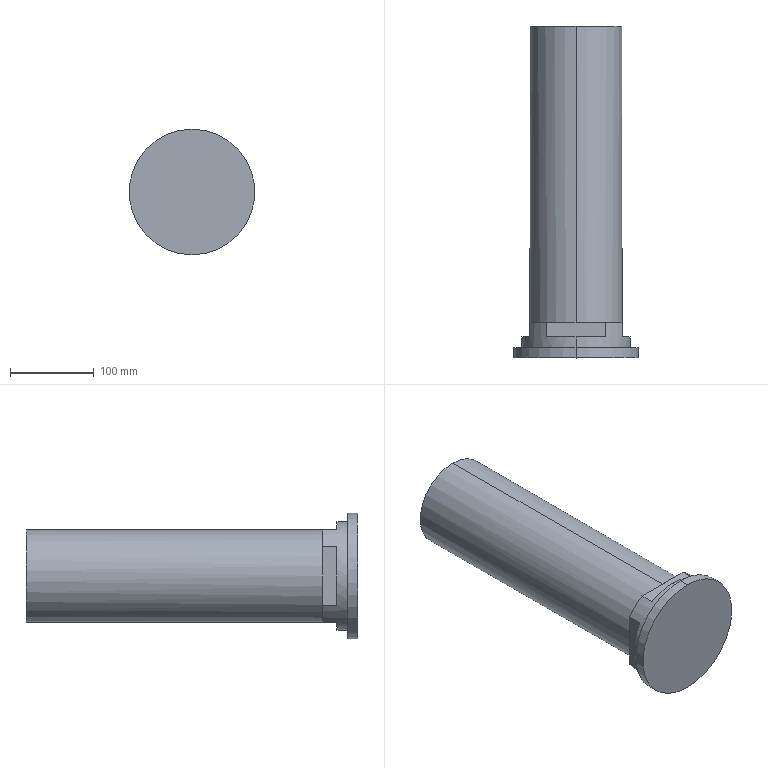Part | SolidWorks | features ICE 4, BaseBody 1 | 1 solid | 21 faces | box 150 x 396 x 150 mm | volume 3942504 mm3 | plane 15 | cylinder 6 | commonest cylinder face diameters 110 x2 130 x2 150 x2
STEP:
#1=CARTESIAN_POINT('',(0.,25.,65.));
#2=VERTEX_POINT('',#1);
#3=CARTESIAN_POINT('',(34.641,25.,55.));
#4=VERTEX_POINT('',#3);
#5=CARTESIAN_POINT('',(0.,25.,0.));
#6=DIRECTION('',(0.,1.,0.));
#7=DIRECTION('',(0.,0.,1.));
#8=AXIS2_PLACEMENT_3D('',#5,#6,#7);
#9=CIRCLE('',#8,65.);
#10=EDGE_CURVE('',#2,#4,#9,.T.);
#11=ORIENTED_EDGE('',*,*,#10,.F.);
#12=CARTESIAN_POINT('',(0.,12.,65.));
#13=VERTEX_POINT('',#12);
#14=CARTESIAN_POINT('',(0.,208.848,65.));
#15=DIRECTION('',(0.,-1.,0.));
#16=VECTOR('',#15,1000.);
#17=LINE('',#14,#16);
#18=EDGE_CURVE('',#2,#13,#17,.T.);
#19=ORIENTED_EDGE('',*,*,#18,.T.);
#20=CARTESIAN_POINT('',(0.,12.,-65.));
#21=VERTEX_POINT('',#20);
#22=CARTESIAN_POINT('',(0.,12.,0.));
#23=DIRECTION('',(0.,1.,0.));
#24=DIRECTION('',(0.,0.,1.));
#25=AXIS2_PLACEMENT_3D('',#22,#23,#24);
#26=CIRCLE('',#25,65.);
#27=EDGE_CURVE('',#13,#21,#26,.T.);
#28=ORIENTED_EDGE('',*,*,#27,.T.);
#29=CARTESIAN_POINT('',(0.,25.,-65.));
#30=VERTEX_POINT('',#29);
#31=CARTESIAN_POINT('',(0.,208.848,-65.));
#32=DIRECTION('',(0.,-1.,0.));
#33=VECTOR('',#32,1000.);
#34=LINE('',#31,#33);
#35=EDGE_CURVE('',#30,#21,#34,.T.);
#36=ORIENTED_EDGE('',*,*,#35,.F.);
#37=CARTESIAN_POINT('',(34.641,25.,-55.));
#38=VERTEX_POINT('',#37);
#39=CARTESIAN_POINT('',(0.,25.,0.));
#40=DIRECTION('',(0.,1.,0.));
#41=DIRECTION('',(0.,0.,1.));
#42=AXIS2_PLACEMENT_3D('',#39,#40,#41);
#43=CIRCLE('',#42,65.);
#44=EDGE_CURVE('',#38,#30,#43,.T.);
#45=ORIENTED_EDGE('',*,*,#44,.F.);
#46=CARTESIAN_POINT('',(34.641,42.,-55.));
#47=VERTEX_POINT('',#46);
#48=CARTESIAN_POINT('',(34.641,197.563,-55.));
#49=DIRECTION('',(0.,-1.,0.));
#50=VECTOR('',#49,1000.);
#51=LINE('',#48,#50);
#52=EDGE_CURVE('',#47,#38,#51,.T.);
#53=ORIENTED_EDGE('',*,*,#52,.F.);
#54=CARTESIAN_POINT('',(55.,42.,-34.641));
#55=VERTEX_POINT('',#54);
#56=CARTESIAN_POINT('',(0.,42.,0.));
#57=DIRECTION('',(0.,1.,0.));
#58=DIRECTION('',(0.,0.,1.));
#59=AXIS2_PLACEMENT_3D('',#56,#57,#58);
#60=CIRCLE('',#59,65.);
#61=EDGE_CURVE('',#55,#47,#60,.T.);
#62=ORIENTED_EDGE('',*,*,#61,.F.);
#63=CARTESIAN_POINT('',(55.,25.,-34.641));
#64=VERTEX_POINT('',#63);
#65=CARTESIAN_POINT('',(55.,197.563,-34.641));
#66=DIRECTION('',(0.,-1.,0.));
#67=VECTOR('',#66,1000.);
#68=LINE('',#65,#67);
#69=EDGE_CURVE('',#55,#64,#68,.T.);
#70=ORIENTED_EDGE('',*,*,#69,.T.);
#71=CARTESIAN_POINT('',(55.,25.,34.641));
#72=VERTEX_POINT('',#71);
#73=CARTESIAN_POINT('',(0.,25.,0.));
#74=DIRECTION('',(0.,1.,0.));
#75=DIRECTION('',(0.,0.,1.));
#76=AXIS2_PLACEMENT_3D('',#73,#74,#75);
#77=CIRCLE('',#76,65.);
#78=EDGE_CURVE('',#72,#64,#77,.T.);
#79=ORIENTED_EDGE('',*,*,#78,.F.);
#80=CARTESIAN_POINT('',(55.,42.,34.641));
#81=VERTEX_POINT('',#80);
#82=CARTESIAN_POINT('',(55.,197.563,34.641));
#83=DIRECTION('',(0.,-1.,0.));
#84=VECTOR('',#83,1000.);
#85=LINE('',#82,#84);
#86=EDGE_CURVE('',#81,#72,#85,.T.);
#87=ORIENTED_EDGE('',*,*,#86,.F.);
#88=CARTESIAN_POINT('',(34.641,42.,55.));
#89=VERTEX_POINT('',#88);
#90=CARTESIAN_POINT('',(0.,42.,0.));
#91=DIRECTION('',(0.,1.,0.));
#92=DIRECTION('',(0.,0.,1.));
#93=AXIS2_PLACEMENT_3D('',#90,#91,#92);
#94=CIRCLE('',#93,65.);
#95=EDGE_CURVE('',#89,#81,#94,.T.);
#96=ORIENTED_EDGE('',*,*,#95,.F.);
#97=CARTESIAN_POINT('',(34.641,197.563,55.));
#98=DIRECTION('',(0.,-1.,0.));
#99=VECTOR('',#98,1000.);
#100=LINE('',#97,#99);
#101=EDGE_CURVE('',#89,#4,#100,.T.);
#102=ORIENTED_EDGE('',*,*,#101,.T.);
#103=EDGE_LOOP('',(#11,#19,#28,#36,#45,#53,#62,#70,#79,#87,#96,#102));
#104=FACE_OUTER_BOUND('',#103,.T.);
#105=CARTESIAN_POINT('',(0.,208.848,0.));
#106=DIRECTION('',(0.,-1.,0.));
#107=DIRECTION('',(0.,0.,-1.));
#108=AXIS2_PLACEMENT_3D('',#105,#106,#107);
#109=CYLINDRICAL_SURFACE('',#108,65.);
#110=ADVANCED_FACE('',(#104),#109,.T.);
#111=CARTESIAN_POINT('',(0.,12.,-75.));
#112=VERTEX_POINT('',#111);
#113=CARTESIAN_POINT('',(0.,12.,75.));
#114=VERTEX_POINT('',#113);
#115=CARTESIAN_POINT('',(0.,12.,0.));
#116=DIRECTION('',(0.,-1.,0.));
#117=DIRECTION('',(0.,0.,1.));
#118=AXIS2_PLACEMENT_3D('',#115,#116,#117);
#119=CIRCLE('',#118,75.);
#120=EDGE_CURVE('',#112,#114,#119,.T.);
#121=ORIENTED_EDGE('',*,*,#120,.T.);
#122=CARTESIAN_POINT('',(0.,0.,75.));
#123=VERTEX_POINT('',#122);
#124=CARTESIAN_POINT('',(0.,224.132,75.));
#125=DIRECTION('',(0.,-1.,0.));
#126=VECTOR('',#125,1000.);
#127=LINE('',#124,#126);
#128=EDGE_CURVE('',#114,#123,#127,.T.);
#129=ORIENTED_EDGE('',*,*,#128,.T.);
#130=CARTESIAN_POINT('',(0.,0.,-75.));
#131=VERTEX_POINT('',#130);
#132=CARTESIAN_POINT('',(0.,0.,0.));
#133=DIRECTION('',(0.,-1.,0.));
#134=DIRECTION('',(0.,0.,-1.));
#135=AXIS2_PLACEMENT_3D('',#132,#133,#134);
#136=CIRCLE('',#135,75.);
#137=EDGE_CURVE('',#131,#123,#136,.T.);
#138=ORIENTED_EDGE('',*,*,#137,.F.);
#139=CARTESIAN_POINT('',(0.,224.132,-75.));
#140=DIRECTION('',(0.,-1.,0.));
#141=VECTOR('',#140,1000.);
#142=LINE('',#139,#141);
#143=EDGE_CURVE('',#112,#131,#142,.T.);
#144=ORIENTED_EDGE('',*,*,#143,.F.);
#145=EDGE_LOOP('',(#121,#129,#138,#144));
#146=FACE_OUTER_BOUND('',#145,.T.);
#147=CARTESIAN_POINT('',(0.,224.132,0.));
#148=DIRECTION('',(0.,-1.,0.));
#149=DIRECTION('',(0.,0.,-1.));
#150=AXIS2_PLACEMENT_3D('',#147,#148,#149);
#151=CYLINDRICAL_SURFACE('',#150,75.);
#152=ADVANCED_FACE('',(#146),#151,.T.);
#153=CARTESIAN_POINT('',(0.,396.,55.));
#154=VERTEX_POINT('',#153);
#155=CARTESIAN_POINT('',(0.,396.,-55.));
#156=VERTEX_POINT('',#155);
#157=CARTESIAN_POINT('',(0.,396.,0.));
#158=DIRECTION('',(0.,1.,0.));
#159=DIRECTION('',(0.,0.,1.));
#160=AXIS2_PLACEMENT_3D('',#157,#158,#159);
#161=CIRCLE('',#160,55.);
#162=EDGE_CURVE('',#154,#156,#161,.T.);
#163=ORIENTED_EDGE('',*,*,#162,.F.);
#164=CARTESIAN_POINT('',(0.,42.,55.));
#165=VERTEX_POINT('',#164);
#166=CARTESIAN_POINT('',(0.,396.,55.));
#167=DIRECTION('',(0.,-1.,0.));
#168=VECTOR('',#167,1000.);
#169=LINE('',#166,#168);
#170=EDGE_CURVE('',#154,#165,#169,.T.);
#171=ORIENTED_EDGE('',*,*,#170,.T.);
#172=CARTESIAN_POINT('',(55.,42.,0.));
#173=VERTEX_POINT('',#172);
#174=CARTESIAN_POINT('',(0.,42.,0.));
#175=DIRECTION('',(0.,1.,0.));
#176=DIRECTION('',(0.,0.,1.));
#177=AXIS2_PLACEMENT_3D('',#174,#175,#176);
#178=CIRCLE('',#177,55.);
#179=EDGE_CURVE('',#165,#173,#178,.T.);
#180=ORIENTED_EDGE('',*,*,#179,.T.);
#181=CARTESIAN_POINT('',(0.,42.,-55.));
#182=VERTEX_POINT('',#181);
#183=CARTESIAN_POINT('',(0.,42.,0.));
#184=DIRECTION('',(0.,1.,0.));
#185=DIRECTION('',(0.,0.,1.));
#186=AXIS2_PLACEMENT_3D('',#183,#184,#185);
#187=CIRCLE('',#186,55.);
#188=EDGE_CURVE('',#173,#182,#187,.T.);
#189=ORIENTED_EDGE('',*,*,#188,.T.);
#190=CARTESIAN_POINT('',(0.,396.,-55.));
#191=DIRECTION('',(0.,-1.,0.));
#192=VECTOR('',#191,1000.);
#193=LINE('',#190,#192);
#194=EDGE_CURVE('',#156,#182,#193,.T.);
#195=ORIENTED_EDGE('',*,*,#194,.F.);
#196=EDGE_LOOP('',(#163,#171,#180,#189,#195));
#197=FACE_OUTER_BOUND('',#196,.T.);
#198=CARTESIAN_POINT('',(0.,396.,0.));
#199=DIRECTION('',(0.,-1.,0.));
#200=DIRECTION('',(0.,0.,-1.));
#201=AXIS2_PLACEMENT_3D('',#198,#199,#200);
#202=CYLINDRICAL_SURFACE('',#201,55.);
#203=ADVANCED_FACE('',(#197),#202,.T.);
#204=ORIENTED_EDGE('',*,*,#170,.F.);
#205=CARTESIAN_POINT('',(0.,396.,0.));
#206=DIRECTION('',(0.,1.,0.));
#207=DIRECTION('',(0.,0.,1.));
#208=AXIS2_PLACEMENT_3D('',#205,#206,#207);
#209=CIRCLE('',#208,55.);
#210=EDGE_CURVE('',#156,#154,#209,.T.);
#211=ORIENTED_EDGE('',*,*,#210,.F.);
#212=ORIENTED_EDGE('',*,*,#194,.T.);
#213=CARTESIAN_POINT('',(-55.,42.,0.));
#214=VERTEX_POINT('',#213);
#215=CARTESIAN_POINT('',(0.,42.,0.));
#216=DIRECTION('',(0.,1.,0.));
#217=DIRECTION('',(0.,0.,1.));
#218=AXIS2_PLACEMENT_3D('',#215,#216,#217);
#219=CIRCLE('',#218,55.);
#220=EDGE_CURVE('',#182,#214,#219,.T.);
#221=ORIENTED_EDGE('',*,*,#220,.T.);
#222=CARTESIAN_POINT('',(0.,42.,0.));
#223=DIRECTION('',(0.,1.,0.));
#224=DIRECTION('',(0.,0.,1.));
#225=AXIS2_PLACEMENT_3D('',#222,#223,#224);
#226=CIRCLE('',#225,55.);
#227=EDGE_CURVE('',#214,#165,#226,.T.);
#228=ORIENTED_EDGE('',*,*,#227,.T.);
#229=EDGE_LOOP('',(#204,#211,#212,#221,#228));
#230=FACE_OUTER_BOUND('',#229,.T.);
#231=CARTESIAN_POINT('',(0.,396.,0.));
#232=DIRECTION('',(0.,-1.,0.));
#233=DIRECTION('',(0.,0.,-1.));
#234=AXIS2_PLACEMENT_3D('',#231,#232,#233);
#235=CYLINDRICAL_SURFACE('',#234,55.);
#236=ADVANCED_FACE('',(#230),#235,.T.);
#237=ORIENTED_EDGE('',*,*,#210,.T.);
#238=ORIENTED_EDGE('',*,*,#162,.T.);
#239=EDGE_LOOP('',(#237,#238));
#240=FACE_OUTER_BOUND('',#239,.T.);
#241=CARTESIAN_POINT('',(0.,396.,0.));
#242=DIRECTION('',(0.,1.,0.));
#243=DIRECTION('',(0.,0.,1.));
#244=AXIS2_PLACEMENT_3D('',#241,#242,#243);
#245=PLANE('',#244);
#246=ADVANCED_FACE('',(#240),#245,.T.);
#247=CARTESIAN_POINT('',(-34.641,42.,55.));
#248=VERTEX_POINT('',#247);
#249=CARTESIAN_POINT('',(-34.641,42.,55.));
#250=DIRECTION('',(1.,0.,0.));
#251=VECTOR('',#250,1000.);
#252=LINE('',#249,#251);
#253=EDGE_CURVE('',#248,#165,#252,.T.);
#254=ORIENTED_EDGE('',*,*,#253,.T.);
#255=ORIENTED_EDGE('',*,*,#227,.F.);
#256=CARTESIAN_POINT('',(-55.,42.,34.641));
#257=VERTEX_POINT('',#256);
#258=CARTESIAN_POINT('',(-55.,42.,34.641));
#259=DIRECTION('',(0.,0.,1.));
#260=VECTOR('',#259,1000.);
#261=LINE('',#258,#260);
#262=EDGE_CURVE('',#214,#257,#261,.T.);
#263=ORIENTED_EDGE('',*,*,#262,.T.);
#264=CARTESIAN_POINT('',(0.,42.,0.));
#265=DIRECTION('',(0.,1.,0.));
#266=DIRECTION('',(0.,0.,1.));
#267=AXIS2_PLACEMENT_3D('',#264,#265,#266);
#268=CIRCLE('',#267,65.);
#269=EDGE_CURVE('',#257,#248,#268,.T.);
#270=ORIENTED_EDGE('',*,*,#269,.T.);
#271=EDGE_LOOP('',(#254,#255,#263,#270));
#272=FACE_OUTER_BOUND('',#271,.T.);
#273=CARTESIAN_POINT('',(0.,42.,0.));
#274=DIRECTION('',(0.,1.,0.));
#275=DIRECTION('',(0.,0.,1.));
#276=AXIS2_PLACEMENT_3D('',#273,#274,#275);
#277=PLANE('',#276);
#278=ADVANCED_FACE('',(#272),#277,.T.);
#279=CARTESIAN_POINT('',(-55.,42.,-34.641));
#280=VERTEX_POINT('',#279);
#281=CARTESIAN_POINT('',(-55.,42.,34.641));
#282=DIRECTION('',(0.,0.,1.));
#283=VECTOR('',#282,1000.);
#284=LINE('',#281,#283);
#285=EDGE_CURVE('',#280,#214,#284,.T.);
#286=ORIENTED_EDGE('',*,*,#285,.T.);
#287=ORIENTED_EDGE('',*,*,#220,.F.);
#288=CARTESIAN_POINT('',(-34.641,42.,-55.));
#289=VERTEX_POINT('',#288);
#290=CARTESIAN_POINT('',(-34.641,42.,-55.));
#291=DIRECTION('',(-1.,0.,0.));
#292=VECTOR('',#291,1000.);
#293=LINE('',#290,#292);
#294=EDGE_CURVE('',#182,#289,#293,.T.);
#295=ORIENTED_EDGE('',*,*,#294,.T.);
#296=CARTESIAN_POINT('',(0.,42.,0.));
#297=DIRECTION('',(0.,1.,0.));
#298=DIRECTION('',(0.,0.,1.));
#299=AXIS2_PLACEMENT_3D('',#296,#297,#298);
#300=CIRCLE('',#299,65.);
#301=EDGE_CURVE('',#289,#280,#300,.T.);
#302=ORIENTED_EDGE('',*,*,#301,.T.);
#303=EDGE_LOOP('',(#286,#287,#295,#302));
#304=FACE_OUTER_BOUND('',#303,.T.);
#305=CARTESIAN_POINT('',(0.,42.,0.));
#306=DIRECTION('',(0.,1.,0.));
#307=DIRECTION('',(0.,0.,1.));
#308=AXIS2_PLACEMENT_3D('',#305,#306,#307);
#309=PLANE('',#308);
#310=ADVANCED_FACE('',(#304),#309,.T.);
#311=CARTESIAN_POINT('',(-34.641,42.,-55.));
#312=DIRECTION('',(-1.,0.,0.));
#313=VECTOR('',#312,1000.);
#314=LINE('',#311,#313);
#315=EDGE_CURVE('',#47,#182,#314,.T.);
#316=ORIENTED_EDGE('',*,*,#315,.T.);
#317=ORIENTED_EDGE('',*,*,#188,.F.);
#318=CARTESIAN_POINT('',(55.,42.,34.641));
#319=DIRECTION('',(0.,0.,-1.));
#320=VECTOR('',#319,1000.);
#321=LINE('',#318,#320);
#322=EDGE_CURVE('',#173,#55,#321,.T.);
#323=ORIENTED_EDGE('',*,*,#322,.T.);
#324=ORIENTED_EDGE('',*,*,#61,.T.);
#325=EDGE_LOOP('',(#316,#317,#323,#324));
#326=FACE_OUTER_BOUND('',#325,.T.);
#327=CARTESIAN_POINT('',(0.,42.,0.));
#328=DIRECTION('',(0.,1.,0.));
#329=DIRECTION('',(0.,0.,1.));
#330=AXIS2_PLACEMENT_3D('',#327,#328,#329);
#331=PLANE('',#330);
#332=ADVANCED_FACE('',(#326),#331,.T.);
#333=CARTESIAN_POINT('',(55.,42.,34.641));
#334=DIRECTION('',(0.,0.,-1.));
#335=VECTOR('',#334,1000.);
#336=LINE('',#333,#335);
#337=EDGE_CURVE('',#81,#173,#336,.T.);
#338=ORIENTED_EDGE('',*,*,#337,.T.);
#339=ORIENTED_EDGE('',*,*,#179,.F.);
#340=CARTESIAN_POINT('',(-34.641,42.,55.));
#341=DIRECTION('',(1.,0.,0.));
#342=VECTOR('',#341,1000.);
#343=LINE('',#340,#342);
#344=EDGE_CURVE('',#165,#89,#343,.T.);
#345=ORIENTED_EDGE('',*,*,#344,.T.);
#346=ORIENTED_EDGE('',*,*,#95,.T.);
#347=EDGE_LOOP('',(#338,#339,#345,#346));
#348=FACE_OUTER_BOUND('',#347,.T.);
#349=CARTESIAN_POINT('',(0.,42.,0.));
#350=DIRECTION('',(0.,1.,0.));
#351=DIRECTION('',(0.,0.,1.));
#352=AXIS2_PLACEMENT_3D('',#349,#350,#351);
#353=PLANE('',#352);
#354=ADVANCED_FACE('',(#348),#353,.T.);
#355=ORIENTED_EDGE('',*,*,#285,.F.);
#356=CARTESIAN_POINT('',(-55.,25.,-34.641));
#357=VERTEX_POINT('',#356);
#358=CARTESIAN_POINT('',(-55.,197.563,-34.641));
#359=DIRECTION('',(0.,-1.,0.));
#360=VECTOR('',#359,1000.);
#361=LINE('',#358,#360);
#362=EDGE_CURVE('',#280,#357,#361,.T.);
#363=ORIENTED_EDGE('',*,*,#362,.T.);
#364=CARTESIAN_POINT('',(-55.,25.,34.641));
#365=VERTEX_POINT('',#364);
#366=CARTESIAN_POINT('',(-55.,25.,34.641));
#367=DIRECTION('',(0.,0.,1.));
#368=VECTOR('',#367,1000.);
#369=LINE('',#366,#368);
#370=EDGE_CURVE('',#357,#365,#369,.T.);
#371=ORIENTED_EDGE('',*,*,#370,.T.);
#372=CARTESIAN_POINT('',(-55.,197.563,34.641));
#373=DIRECTION('',(0.,-1.,0.));
#374=VECTOR('',#373,1000.);
#375=LINE('',#372,#374);
#376=EDGE_CURVE('',#257,#365,#375,.T.);
#377=ORIENTED_EDGE('',*,*,#376,.F.);
#378=ORIENTED_EDGE('',*,*,#262,.F.);
#379=EDGE_LOOP('',(#355,#363,#371,#377,#378));
#380=FACE_OUTER_BOUND('',#379,.T.);
#381=CARTESIAN_POINT('',(-55.,197.563,34.641));
#382=DIRECTION('',(1.,0.,0.));
#383=DIRECTION('',(0.,0.,-1.));
#384=AXIS2_PLACEMENT_3D('',#381,#382,#383);
#385=PLANE('',#384);
#386=ADVANCED_FACE('',(#380),#385,.F.);
#387=ORIENTED_EDGE('',*,*,#253,.F.);
#388=CARTESIAN_POINT('',(-34.641,25.,55.));
#389=VERTEX_POINT('',#388);
#390=CARTESIAN_POINT('',(-34.641,197.563,55.));
#391=DIRECTION('',(0.,-1.,0.));
#392=VECTOR('',#391,1000.);
#393=LINE('',#390,#392);
#394=EDGE_CURVE('',#248,#389,#393,.T.);
#395=ORIENTED_EDGE('',*,*,#394,.T.);
#396=CARTESIAN_POINT('',(-34.641,25.,55.));
#397=DIRECTION('',(1.,0.,0.));
#398=VECTOR('',#397,1000.);
#399=LINE('',#396,#398);
#400=EDGE_CURVE('',#389,#4,#399,.T.);
#401=ORIENTED_EDGE('',*,*,#400,.T.);
#402=ORIENTED_EDGE('',*,*,#101,.F.);
#403=ORIENTED_EDGE('',*,*,#344,.F.);
#404=EDGE_LOOP('',(#387,#395,#401,#402,#403));
#405=FACE_OUTER_BOUND('',#404,.T.);
#406=CARTESIAN_POINT('',(-34.641,197.563,55.));
#407=DIRECTION('',(0.,0.,-1.));
#408=DIRECTION('',(-1.,0.,0.));
#409=AXIS2_PLACEMENT_3D('',#406,#407,#408);
#410=PLANE('',#409);
#411=ADVANCED_FACE('',(#405),#410,.F.);
#412=ORIENTED_EDGE('',*,*,#337,.F.);
#413=ORIENTED_EDGE('',*,*,#86,.T.);
#414=CARTESIAN_POINT('',(55.,25.,34.641));
#415=DIRECTION('',(0.,0.,-1.));
#416=VECTOR('',#415,1000.);
#417=LINE('',#414,#416);
#418=EDGE_CURVE('',#72,#64,#417,.T.);
#419=ORIENTED_EDGE('',*,*,#418,.T.);
#420=ORIENTED_EDGE('',*,*,#69,.F.);
#421=ORIENTED_EDGE('',*,*,#322,.F.);
#422=EDGE_LOOP('',(#412,#413,#419,#420,#421));
#423=FACE_OUTER_BOUND('',#422,.T.);
#424=CARTESIAN_POINT('',(55.,197.563,34.641));
#425=DIRECTION('',(-1.,0.,0.));
#426=DIRECTION('',(0.,0.,1.));
#427=AXIS2_PLACEMENT_3D('',#424,#425,#426);
#428=PLANE('',#427);
#429=ADVANCED_FACE('',(#423),#428,.F.);
#430=ORIENTED_EDGE('',*,*,#315,.F.);
#431=ORIENTED_EDGE('',*,*,#52,.T.);
#432=CARTESIAN_POINT('',(-34.641,25.,-55.));
#433=VERTEX_POINT('',#432);
#434=CARTESIAN_POINT('',(-34.641,25.,-55.));
#435=DIRECTION('',(-1.,0.,0.));
#436=VECTOR('',#435,1000.);
#437=LINE('',#434,#436);
#438=EDGE_CURVE('',#38,#433,#437,.T.);
#439=ORIENTED_EDGE('',*,*,#438,.T.);
#440=CARTESIAN_POINT('',(-34.641,197.563,-55.));
#441=DIRECTION('',(0.,-1.,0.));
#442=VECTOR('',#441,1000.);
#443=LINE('',#440,#442);
#444=EDGE_CURVE('',#289,#433,#443,.T.);
#445=ORIENTED_EDGE('',*,*,#444,.F.);
#446=ORIENTED_EDGE('',*,*,#294,.F.);
#447=EDGE_LOOP('',(#430,#431,#439,#445,#446));
#448=FACE_OUTER_BOUND('',#447,.T.);
#449=CARTESIAN_POINT('',(-34.641,197.563,-55.));
#450=DIRECTION('',(0.,0.,1.));
#451=DIRECTION('',(1.,0.,0.));
#452=AXIS2_PLACEMENT_3D('',#449,#450,#451);
#453=PLANE('',#452);
#454=ADVANCED_FACE('',(#448),#453,.F.);
#455=ORIENTED_EDGE('',*,*,#137,.T.);
#456=CARTESIAN_POINT('',(0.,0.,0.));
#457=DIRECTION('',(0.,-1.,0.));
#458=DIRECTION('',(0.,0.,-1.));
#459=AXIS2_PLACEMENT_3D('',#456,#457,#458);
#460=CIRCLE('',#459,75.);
#461=EDGE_CURVE('',#123,#131,#460,.T.);
#462=ORIENTED_EDGE('',*,*,#461,.T.);
#463=EDGE_LOOP('',(#455,#462));
#464=FACE_OUTER_BOUND('',#463,.T.);
#465=CARTESIAN_POINT('',(0.,0.,0.));
#466=DIRECTION('',(0.,1.,0.));
#467=DIRECTION('',(0.,0.,1.));
#468=AXIS2_PLACEMENT_3D('',#465,#466,#467);
#469=PLANE('',#468);
#470=ADVANCED_FACE('',(#464),#469,.F.);
#471=ORIENTED_EDGE('',*,*,#128,.F.);
#472=CARTESIAN_POINT('',(0.,12.,0.));
#473=DIRECTION('',(0.,-1.,0.));
#474=DIRECTION('',(0.,0.,1.));
#475=AXIS2_PLACEMENT_3D('',#472,#473,#474);
#476=CIRCLE('',#475,75.);
#477=EDGE_CURVE('',#114,#112,#476,.T.);
#478=ORIENTED_EDGE('',*,*,#477,.T.);
#479=ORIENTED_EDGE('',*,*,#143,.T.);
#480=ORIENTED_EDGE('',*,*,#461,.F.);
#481=EDGE_LOOP('',(#471,#478,#479,#480));
#482=FACE_OUTER_BOUND('',#481,.T.);
#483=CARTESIAN_POINT('',(0.,224.132,0.));
#484=DIRECTION('',(0.,-1.,0.));
#485=DIRECTION('',(0.,0.,-1.));
#486=AXIS2_PLACEMENT_3D('',#483,#484,#485);
#487=CYLINDRICAL_SURFACE('',#486,75.);
#488=ADVANCED_FACE('',(#482),#487,.T.);
#489=CARTESIAN_POINT('',(0.,12.,0.));
#490=DIRECTION('',(0.,1.,0.));
#491=DIRECTION('',(0.,0.,1.));
#492=AXIS2_PLACEMENT_3D('',#489,#490,#491);
#493=CIRCLE('',#492,65.);
#494=EDGE_CURVE('',#21,#13,#493,.T.);
#495=ORIENTED_EDGE('',*,*,#494,.F.);
#496=ORIENTED_EDGE('',*,*,#27,.F.);
#497=EDGE_LOOP('',(#495,#496));
#498=FACE_BOUND('',#497,.T.);
#499=ORIENTED_EDGE('',*,*,#120,.F.);
#500=ORIENTED_EDGE('',*,*,#477,.F.);
#501=EDGE_LOOP('',(#499,#500));
#502=FACE_OUTER_BOUND('',#501,.T.);
#503=CARTESIAN_POINT('',(0.,12.,0.));
#504=DIRECTION('',(0.,1.,0.));
#505=DIRECTION('',(0.,0.,1.));
#506=AXIS2_PLACEMENT_3D('',#503,#504,#505);
#507=PLANE('',#506);
#508=ADVANCED_FACE('',(#498,#502),#507,.T.);
#509=ORIENTED_EDGE('',*,*,#18,.F.);
#510=CARTESIAN_POINT('',(0.,25.,0.));
#511=DIRECTION('',(0.,1.,0.));
#512=DIRECTION('',(0.,0.,1.));
#513=AXIS2_PLACEMENT_3D('',#510,#511,#512);
#514=CIRCLE('',#513,65.);
#515=EDGE_CURVE('',#389,#2,#514,.T.);
#516=ORIENTED_EDGE('',*,*,#515,.F.);
#517=ORIENTED_EDGE('',*,*,#394,.F.);
#518=ORIENTED_EDGE('',*,*,#269,.F.);
#519=ORIENTED_EDGE('',*,*,#376,.T.);
#520=CARTESIAN_POINT('',(0.,25.,0.));
#521=DIRECTION('',(0.,1.,0.));
#522=DIRECTION('',(0.,0.,1.));
#523=AXIS2_PLACEMENT_3D('',#520,#521,#522);
#524=CIRCLE('',#523,65.);
#525=EDGE_CURVE('',#357,#365,#524,.T.);
#526=ORIENTED_EDGE('',*,*,#525,.F.);
#527=ORIENTED_EDGE('',*,*,#362,.F.);
#528=ORIENTED_EDGE('',*,*,#301,.F.);
#529=ORIENTED_EDGE('',*,*,#444,.T.);
#530=CARTESIAN_POINT('',(0.,25.,0.));
#531=DIRECTION('',(0.,1.,0.));
#532=DIRECTION('',(0.,0.,1.));
#533=AXIS2_PLACEMENT_3D('',#530,#531,#532);
#534=CIRCLE('',#533,65.);
#535=EDGE_CURVE('',#30,#433,#534,.T.);
#536=ORIENTED_EDGE('',*,*,#535,.F.);
#537=ORIENTED_EDGE('',*,*,#35,.T.);
#538=ORIENTED_EDGE('',*,*,#494,.T.);
#539=EDGE_LOOP('',(#509,#516,#517,#518,#519,#526,#527,#528,#529,#536,#537,#538));
#540=FACE_OUTER_BOUND('',#539,.T.);
#541=CARTESIAN_POINT('',(0.,208.848,0.));
#542=DIRECTION('',(0.,-1.,0.));
#543=DIRECTION('',(0.,0.,-1.));
#544=AXIS2_PLACEMENT_3D('',#541,#542,#543);
#545=CYLINDRICAL_SURFACE('',#544,65.);
#546=ADVANCED_FACE('',(#540),#545,.T.);
#547=ORIENTED_EDGE('',*,*,#44,.T.);
#548=ORIENTED_EDGE('',*,*,#535,.T.);
#549=ORIENTED_EDGE('',*,*,#438,.F.);
#550=EDGE_LOOP('',(#547,#548,#549));
#551=FACE_OUTER_BOUND('',#550,.T.);
#552=CARTESIAN_POINT('',(0.,25.,0.));
#553=DIRECTION('',(0.,1.,0.));
#554=DIRECTION('',(0.,0.,1.));
#555=AXIS2_PLACEMENT_3D('',#552,#553,#554);
#556=PLANE('',#555);
#557=ADVANCED_FACE('',(#551),#556,.T.);
#558=ORIENTED_EDGE('',*,*,#78,.T.);
#559=ORIENTED_EDGE('',*,*,#418,.F.);
#560=EDGE_LOOP('',(#558,#559));
#561=FACE_OUTER_BOUND('',#560,.T.);
#562=CARTESIAN_POINT('',(0.,25.,0.));
#563=DIRECTION('',(0.,1.,0.));
#564=DIRECTION('',(0.,0.,1.));
#565=AXIS2_PLACEMENT_3D('',#562,#563,#564);
#566=PLANE('',#565);
#567=ADVANCED_FACE('',(#561),#566,.T.);
#568=ORIENTED_EDGE('',*,*,#515,.T.);
#569=ORIENTED_EDGE('',*,*,#10,.T.);
#570=ORIENTED_EDGE('',*,*,#400,.F.);
#571=EDGE_LOOP('',(#568,#569,#570));
#572=FACE_OUTER_BOUND('',#571,.T.);
#573=CARTESIAN_POINT('',(0.,25.,0.));
#574=DIRECTION('',(0.,1.,0.));
#575=DIRECTION('',(0.,0.,1.));
#576=AXIS2_PLACEMENT_3D('',#573,#574,#575);
#577=PLANE('',#576);
#578=ADVANCED_FACE('',(#572),#577,.T.);
#579=ORIENTED_EDGE('',*,*,#525,.T.);
#580=ORIENTED_EDGE('',*,*,#370,.F.);
#581=EDGE_LOOP('',(#579,#580));
#582=FACE_OUTER_BOUND('',#581,.T.);
#583=CARTESIAN_POINT('',(0.,25.,0.));
#584=DIRECTION('',(0.,1.,0.));
#585=DIRECTION('',(0.,0.,1.));
#586=AXIS2_PLACEMENT_3D('',#583,#584,#585);
#587=PLANE('',#586);
#588=ADVANCED_FACE('',(#582),#587,.T.);
#589=CLOSED_SHELL('',(#110,#152,#203,#236,#246,#278,#310,#332,#354,#386,#411,#429,#454,#470,#488,#508,#546,#557,#567,#578,#588));
#590=MANIFOLD_SOLID_BREP('',#589);
#591=CARTESIAN_POINT('',(0.,0.,0.));
#592=DIRECTION('',(0.,0.,1.));
#593=DIRECTION('',(1.,0.,0.));
#594=AXIS2_PLACEMENT_3D('',#591,#592,#593);
#595=(LENGTH_UNIT()NAMED_UNIT(*)SI_UNIT(.MILLI.,.METRE.));
#596=UNCERTAINTY_MEASURE_WITH_UNIT(LENGTH_MEASURE(0.00001),#595,'','');
#597=(NAMED_UNIT(*)PLANE_ANGLE_UNIT()SI_UNIT($,.RADIAN.));
#598=(NAMED_UNIT(*)SI_UNIT($,.STERADIAN.)SOLID_ANGLE_UNIT());
#599=(GEOMETRIC_REPRESENTATION_CONTEXT(3)GLOBAL_UNCERTAINTY_ASSIGNED_CONTEXT((#596))GLOBAL_UNIT_ASSIGNED_CONTEXT((#595,#597,#598))REPRESENTATION_CONTEXT('',''));
#600=ADVANCED_BREP_SHAPE_REPRESENTATION('',(#590,#594),#599);